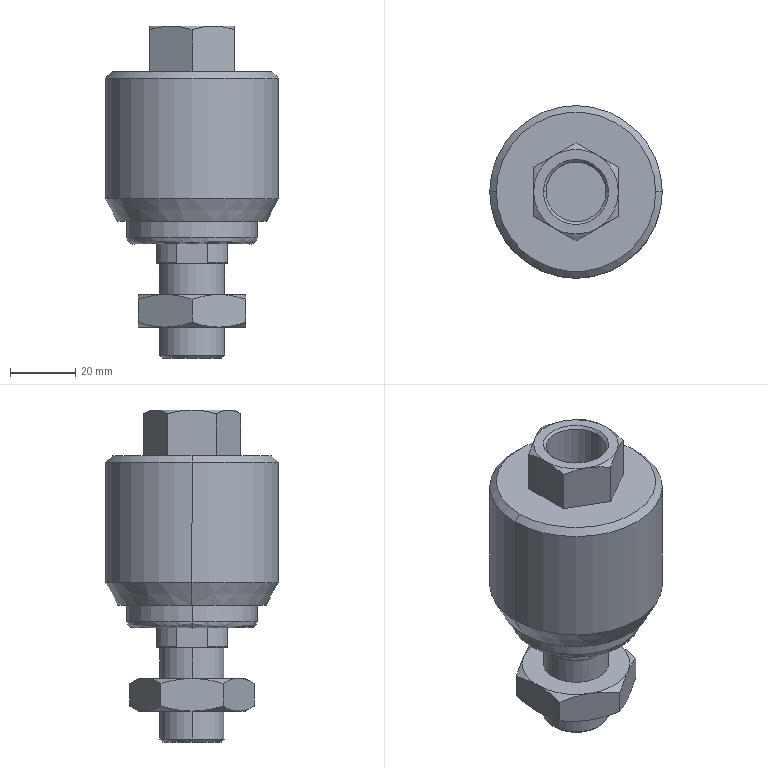Part | SolidWorks | features BaseBody 1 | 1 solid | 82 faces | box 53 x 53 x 102 mm | volume 127493 mm3 | cone 38 | plane 28 | cylinder 14 | spline 2 | commonest cylinder face diameters 20 x4 24 x4 18.376 x2 40 x2 53 x2